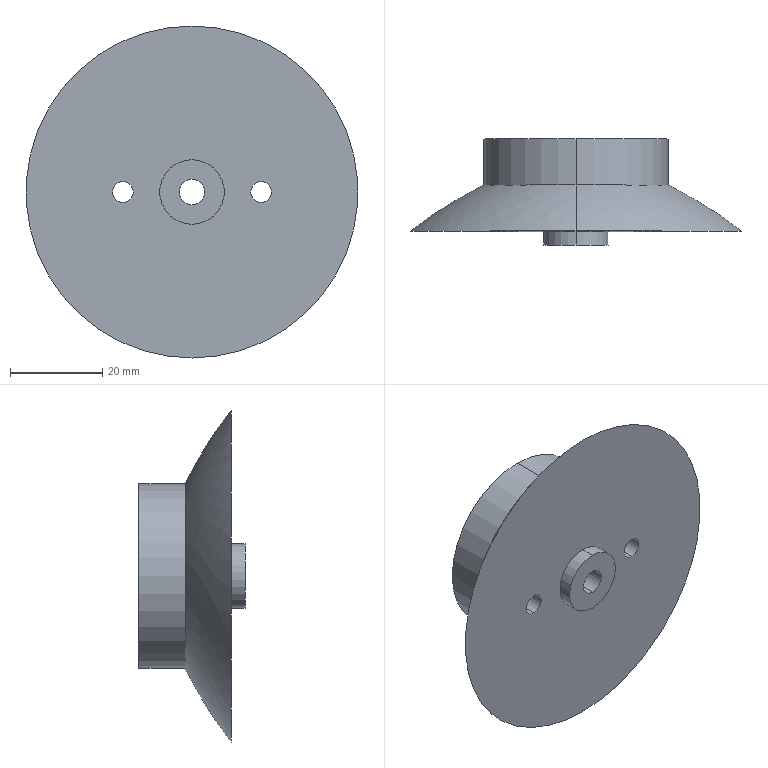Part | STEP file | Motor pulley PTFE pressure pad SGN-4-11 | 1 solid | 24 faces | box 72 x 23 x 72 mm | volume 37619 mm3 | cylinder 16 | plane 6 | other 2 | commonest cylinder face diameters 4.5 x4 8 x4 5.5 x2 10 x2 14 x2 40 x2